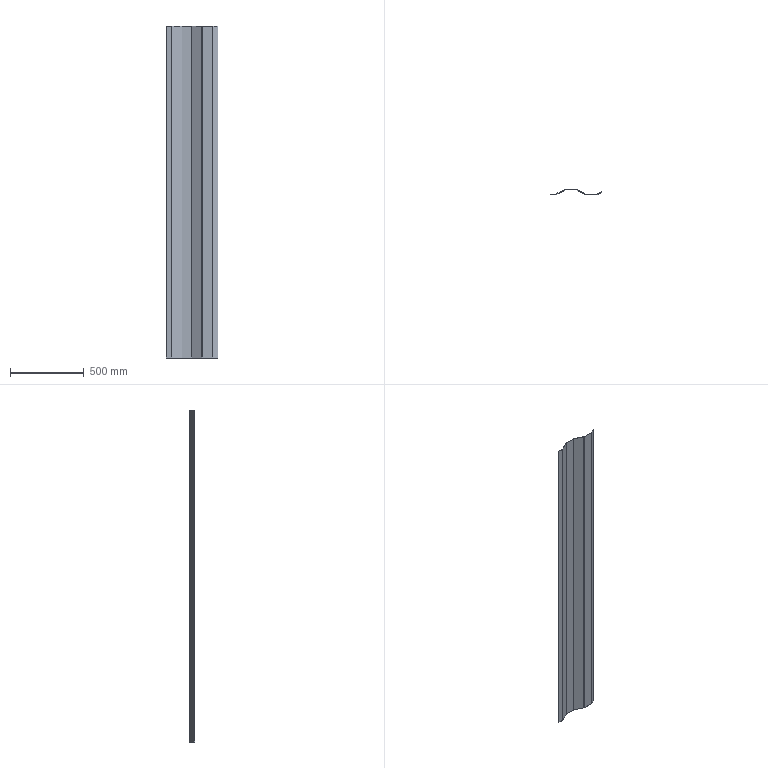Part | STEP file | 750078174 | 1 solid | 26 faces | box 347 x 36 x 2253 mm | volume 1650208 mm3 | plane 16 | cylinder 10 | commonest cylinder face diameters 6 x5 10 x5
STEP:
#1=CARTESIAN_POINT('',(102.472,35.472,0.));
#2=VERTEX_POINT('',#1);
#3=CARTESIAN_POINT('',(36.161,2.317,0.));
#4=VERTEX_POINT('',#3);
#5=CARTESIAN_POINT('',(103.106,35.789,0.));
#6=DIRECTION('',(-0.8944,-0.4472,0.));
#7=VECTOR('',#6,1000.);
#8=LINE('',#5,#7);
#9=EDGE_CURVE('',#2,#4,#8,.T.);
#10=ORIENTED_EDGE('',*,*,#9,.T.);
#11=CARTESIAN_POINT('',(36.161,2.317,2252.5));
#12=VERTEX_POINT('',#11);
#13=CARTESIAN_POINT('',(36.161,2.317,0.));
#14=DIRECTION('',(0.,0.,1.));
#15=VECTOR('',#14,1000.);
#16=LINE('',#13,#15);
#17=EDGE_CURVE('',#4,#12,#16,.T.);
#18=ORIENTED_EDGE('',*,*,#17,.T.);
#19=CARTESIAN_POINT('',(102.472,35.472,2252.5));
#20=VERTEX_POINT('',#19);
#21=CARTESIAN_POINT('',(103.106,35.789,2252.5));
#22=DIRECTION('',(0.8944,0.4472,0.));
#23=VECTOR('',#22,1000.);
#24=LINE('',#21,#23);
#25=EDGE_CURVE('',#12,#20,#24,.T.);
#26=ORIENTED_EDGE('',*,*,#25,.T.);
#27=CARTESIAN_POINT('',(102.472,35.472,0.));
#28=DIRECTION('',(0.,0.,-1.));
#29=VECTOR('',#28,1000.);
#30=LINE('',#27,#29);
#31=EDGE_CURVE('',#20,#2,#30,.T.);
#32=ORIENTED_EDGE('',*,*,#31,.T.);
#33=EDGE_LOOP('',(#10,#18,#26,#32));
#34=FACE_OUTER_BOUND('',#33,.T.);
#35=CARTESIAN_POINT('',(103.106,35.789,0.));
#36=DIRECTION('',(-0.4472,0.8944,0.));
#37=DIRECTION('',(-0.8944,-0.4472,0.));
#38=AXIS2_PLACEMENT_3D('',#35,#36,#37);
#39=PLANE('',#38);
#40=ADVANCED_FACE('',(#34),#39,.T.);
#41=ORIENTED_EDGE('',*,*,#17,.F.);
#42=CARTESIAN_POINT('',(34.82,2.,0.));
#43=VERTEX_POINT('',#42);
#44=CARTESIAN_POINT('',(34.82,5.,0.));
#45=DIRECTION('',(0.,0.,1.));
#46=DIRECTION('',(1.,0.,0.));
#47=AXIS2_PLACEMENT_3D('',#44,#45,#46);
#48=CIRCLE('',#47,3.);
#49=EDGE_CURVE('',#43,#4,#48,.T.);
#50=ORIENTED_EDGE('',*,*,#49,.F.);
#51=CARTESIAN_POINT('',(34.82,2.,2252.5));
#52=VERTEX_POINT('',#51);
#53=CARTESIAN_POINT('',(34.82,2.,0.));
#54=DIRECTION('',(0.,0.,-1.));
#55=VECTOR('',#54,1000.);
#56=LINE('',#53,#55);
#57=EDGE_CURVE('',#52,#43,#56,.T.);
#58=ORIENTED_EDGE('',*,*,#57,.F.);
#59=CARTESIAN_POINT('',(34.82,5.,2252.5));
#60=DIRECTION('',(0.,0.,-1.));
#61=DIRECTION('',(1.,0.,0.));
#62=AXIS2_PLACEMENT_3D('',#59,#60,#61);
#63=CIRCLE('',#62,3.);
#64=EDGE_CURVE('',#12,#52,#63,.T.);
#65=ORIENTED_EDGE('',*,*,#64,.F.);
#66=EDGE_LOOP('',(#41,#50,#58,#65));
#67=FACE_OUTER_BOUND('',#66,.T.);
#68=CARTESIAN_POINT('',(34.82,5.,0.));
#69=DIRECTION('',(0.,0.,1.));
#70=DIRECTION('',(1.,0.,0.));
#71=AXIS2_PLACEMENT_3D('',#68,#69,#70);
#72=CYLINDRICAL_SURFACE('',#71,3.);
#73=ADVANCED_FACE('',(#67),#72,.F.);
#74=CARTESIAN_POINT('',(314.161,2.317,0.));
#75=VERTEX_POINT('',#74);
#76=CARTESIAN_POINT('',(346.106,18.289,0.));
#77=VERTEX_POINT('',#76);
#78=CARTESIAN_POINT('',(314.161,2.317,0.));
#79=DIRECTION('',(0.8944,0.4472,0.));
#80=VECTOR('',#79,1000.);
#81=LINE('',#78,#80);
#82=EDGE_CURVE('',#75,#77,#81,.T.);
#83=ORIENTED_EDGE('',*,*,#82,.T.);
#84=CARTESIAN_POINT('',(347.,16.5,0.));
#85=VERTEX_POINT('',#84);
#86=CARTESIAN_POINT('',(346.106,18.289,0.));
#87=DIRECTION('',(0.4472,-0.8944,0.));
#88=VECTOR('',#87,1000.);
#89=LINE('',#86,#88);
#90=EDGE_CURVE('',#77,#85,#89,.T.);
#91=ORIENTED_EDGE('',*,*,#90,.T.);
#92=CARTESIAN_POINT('',(315.056,0.5279,0.));
#93=VERTEX_POINT('',#92);
#94=CARTESIAN_POINT('',(347.,16.5,0.));
#95=DIRECTION('',(-0.8944,-0.4472,0.));
#96=VECTOR('',#95,1000.);
#97=LINE('',#94,#96);
#98=EDGE_CURVE('',#85,#93,#97,.T.);
#99=ORIENTED_EDGE('',*,*,#98,.T.);
#100=CARTESIAN_POINT('',(312.82,0.,0.));
#101=VERTEX_POINT('',#100);
#102=CARTESIAN_POINT('',(312.82,5.,0.));
#103=DIRECTION('',(0.,0.,-1.));
#104=DIRECTION('',(1.,0.,0.));
#105=AXIS2_PLACEMENT_3D('',#102,#103,#104);
#106=CIRCLE('',#105,5.);
#107=EDGE_CURVE('',#93,#101,#106,.T.);
#108=ORIENTED_EDGE('',*,*,#107,.T.);
#109=CARTESIAN_POINT('',(243.18,0.,0.));
#110=VERTEX_POINT('',#109);
#111=CARTESIAN_POINT('',(347.,0.,0.));
#112=DIRECTION('',(-1.,0.,0.));
#113=VECTOR('',#112,1000.);
#114=LINE('',#111,#113);
#115=EDGE_CURVE('',#101,#110,#114,.T.);
#116=ORIENTED_EDGE('',*,*,#115,.T.);
#117=CARTESIAN_POINT('',(240.944,0.5279,0.));
#118=VERTEX_POINT('',#117);
#119=CARTESIAN_POINT('',(243.18,5.,0.));
#120=DIRECTION('',(0.,0.,-1.));
#121=DIRECTION('',(1.,0.,0.));
#122=AXIS2_PLACEMENT_3D('',#119,#120,#121);
#123=CIRCLE('',#122,5.);
#124=EDGE_CURVE('',#110,#118,#123,.T.);
#125=ORIENTED_EDGE('',*,*,#124,.T.);
#126=CARTESIAN_POINT('',(174.633,33.683,0.));
#127=VERTEX_POINT('',#126);
#128=CARTESIAN_POINT('',(240.944,0.5279,0.));
#129=DIRECTION('',(-0.8944,0.4472,0.));
#130=VECTOR('',#129,1000.);
#131=LINE('',#128,#130);
#132=EDGE_CURVE('',#118,#127,#131,.T.);
#133=ORIENTED_EDGE('',*,*,#132,.T.);
#134=CARTESIAN_POINT('',(173.292,34.,0.));
#135=VERTEX_POINT('',#134);
#136=CARTESIAN_POINT('',(173.292,31.,0.));
#137=DIRECTION('',(0.,0.,1.));
#138=DIRECTION('',(1.,0.,0.));
#139=AXIS2_PLACEMENT_3D('',#136,#137,#138);
#140=CIRCLE('',#139,3.);
#141=EDGE_CURVE('',#127,#135,#140,.T.);
#142=ORIENTED_EDGE('',*,*,#141,.T.);
#143=CARTESIAN_POINT('',(104.708,34.,0.));
#144=VERTEX_POINT('',#143);
#145=CARTESIAN_POINT('',(347.,34.,0.));
#146=DIRECTION('',(-1.,0.,0.));
#147=VECTOR('',#146,1000.);
#148=LINE('',#145,#147);
#149=EDGE_CURVE('',#135,#144,#148,.T.);
#150=ORIENTED_EDGE('',*,*,#149,.T.);
#151=CARTESIAN_POINT('',(103.367,33.683,0.));
#152=VERTEX_POINT('',#151);
#153=CARTESIAN_POINT('',(104.708,31.,0.));
#154=DIRECTION('',(0.,0.,1.));
#155=DIRECTION('',(1.,0.,0.));
#156=AXIS2_PLACEMENT_3D('',#153,#154,#155);
#157=CIRCLE('',#156,3.);
#158=EDGE_CURVE('',#144,#152,#157,.T.);
#159=ORIENTED_EDGE('',*,*,#158,.T.);
#160=CARTESIAN_POINT('',(37.056,0.5279,0.));
#161=VERTEX_POINT('',#160);
#162=CARTESIAN_POINT('',(103.367,33.683,0.));
#163=DIRECTION('',(-0.8944,-0.4472,0.));
#164=VECTOR('',#163,1000.);
#165=LINE('',#162,#164);
#166=EDGE_CURVE('',#152,#161,#165,.T.);
#167=ORIENTED_EDGE('',*,*,#166,.T.);
#168=CARTESIAN_POINT('',(34.82,0.,0.));
#169=VERTEX_POINT('',#168);
#170=CARTESIAN_POINT('',(34.82,5.,0.));
#171=DIRECTION('',(0.,0.,-1.));
#172=DIRECTION('',(1.,0.,0.));
#173=AXIS2_PLACEMENT_3D('',#170,#171,#172);
#174=CIRCLE('',#173,5.);
#175=EDGE_CURVE('',#161,#169,#174,.T.);
#176=ORIENTED_EDGE('',*,*,#175,.T.);
#177=CARTESIAN_POINT('',(0.,0.,0.));
#178=VERTEX_POINT('',#177);
#179=CARTESIAN_POINT('',(347.,0.,0.));
#180=DIRECTION('',(-1.,0.,0.));
#181=VECTOR('',#180,1000.);
#182=LINE('',#179,#181);
#183=EDGE_CURVE('',#169,#178,#182,.T.);
#184=ORIENTED_EDGE('',*,*,#183,.T.);
#185=CARTESIAN_POINT('',(0.,2.,0.));
#186=VERTEX_POINT('',#185);
#187=CARTESIAN_POINT('',(0.,16.5,0.));
#188=DIRECTION('',(0.,1.,0.));
#189=VECTOR('',#188,1000.);
#190=LINE('',#187,#189);
#191=EDGE_CURVE('',#178,#186,#190,.T.);
#192=ORIENTED_EDGE('',*,*,#191,.T.);
#193=CARTESIAN_POINT('',(347.,2.,0.));
#194=DIRECTION('',(1.,0.,0.));
#195=VECTOR('',#194,1000.);
#196=LINE('',#193,#195);
#197=EDGE_CURVE('',#186,#43,#196,.T.);
#198=ORIENTED_EDGE('',*,*,#197,.T.);
#199=ORIENTED_EDGE('',*,*,#49,.T.);
#200=ORIENTED_EDGE('',*,*,#9,.F.);
#201=CARTESIAN_POINT('',(104.708,36.,0.));
#202=VERTEX_POINT('',#201);
#203=CARTESIAN_POINT('',(104.708,31.,0.));
#204=DIRECTION('',(0.,0.,-1.));
#205=DIRECTION('',(1.,0.,0.));
#206=AXIS2_PLACEMENT_3D('',#203,#204,#205);
#207=CIRCLE('',#206,5.);
#208=EDGE_CURVE('',#2,#202,#207,.T.);
#209=ORIENTED_EDGE('',*,*,#208,.T.);
#210=CARTESIAN_POINT('',(173.292,36.,0.));
#211=VERTEX_POINT('',#210);
#212=CARTESIAN_POINT('',(347.,36.,0.));
#213=DIRECTION('',(1.,0.,0.));
#214=VECTOR('',#213,1000.);
#215=LINE('',#212,#214);
#216=EDGE_CURVE('',#202,#211,#215,.T.);
#217=ORIENTED_EDGE('',*,*,#216,.T.);
#218=CARTESIAN_POINT('',(175.528,35.472,0.));
#219=VERTEX_POINT('',#218);
#220=CARTESIAN_POINT('',(173.292,31.,0.));
#221=DIRECTION('',(0.,0.,-1.));
#222=DIRECTION('',(1.,0.,0.));
#223=AXIS2_PLACEMENT_3D('',#220,#221,#222);
#224=CIRCLE('',#223,5.);
#225=EDGE_CURVE('',#211,#219,#224,.T.);
#226=ORIENTED_EDGE('',*,*,#225,.T.);
#227=CARTESIAN_POINT('',(241.839,2.317,0.));
#228=VERTEX_POINT('',#227);
#229=CARTESIAN_POINT('',(175.528,35.472,0.));
#230=DIRECTION('',(0.8944,-0.4472,0.));
#231=VECTOR('',#230,1000.);
#232=LINE('',#229,#231);
#233=EDGE_CURVE('',#219,#228,#232,.T.);
#234=ORIENTED_EDGE('',*,*,#233,.T.);
#235=CARTESIAN_POINT('',(243.18,2.,0.));
#236=VERTEX_POINT('',#235);
#237=CARTESIAN_POINT('',(243.18,5.,0.));
#238=DIRECTION('',(0.,0.,1.));
#239=DIRECTION('',(1.,0.,0.));
#240=AXIS2_PLACEMENT_3D('',#237,#238,#239);
#241=CIRCLE('',#240,3.);
#242=EDGE_CURVE('',#228,#236,#241,.T.);
#243=ORIENTED_EDGE('',*,*,#242,.T.);
#244=CARTESIAN_POINT('',(312.82,2.,0.));
#245=VERTEX_POINT('',#244);
#246=CARTESIAN_POINT('',(347.,2.,0.));
#247=DIRECTION('',(1.,0.,0.));
#248=VECTOR('',#247,1000.);
#249=LINE('',#246,#248);
#250=EDGE_CURVE('',#236,#245,#249,.T.);
#251=ORIENTED_EDGE('',*,*,#250,.T.);
#252=CARTESIAN_POINT('',(312.82,5.,0.));
#253=DIRECTION('',(0.,0.,1.));
#254=DIRECTION('',(1.,0.,0.));
#255=AXIS2_PLACEMENT_3D('',#252,#253,#254);
#256=CIRCLE('',#255,3.);
#257=EDGE_CURVE('',#245,#75,#256,.T.);
#258=ORIENTED_EDGE('',*,*,#257,.T.);
#259=EDGE_LOOP('',(#83,#91,#99,#108,#116,#125,#133,#142,#150,#159,#167,#176,#184,#192,#198,#199,#200,#209,#217,#226,#234,#243,#251,#258));
#260=FACE_OUTER_BOUND('',#259,.T.);
#261=CARTESIAN_POINT('',(347.,16.5,0.));
#262=DIRECTION('',(0.,0.,-1.));
#263=DIRECTION('',(-1.,0.,0.));
#264=AXIS2_PLACEMENT_3D('',#261,#262,#263);
#265=PLANE('',#264);
#266=ADVANCED_FACE('',(#260),#265,.T.);
#267=ORIENTED_EDGE('',*,*,#208,.F.);
#268=ORIENTED_EDGE('',*,*,#31,.F.);
#269=CARTESIAN_POINT('',(104.708,36.,2252.5));
#270=VERTEX_POINT('',#269);
#271=CARTESIAN_POINT('',(104.708,31.,2252.5));
#272=DIRECTION('',(0.,0.,-1.));
#273=DIRECTION('',(1.,0.,0.));
#274=AXIS2_PLACEMENT_3D('',#271,#272,#273);
#275=CIRCLE('',#274,5.);
#276=EDGE_CURVE('',#20,#270,#275,.T.);
#277=ORIENTED_EDGE('',*,*,#276,.T.);
#278=CARTESIAN_POINT('',(104.708,36.,0.));
#279=DIRECTION('',(0.,0.,-1.));
#280=VECTOR('',#279,1000.);
#281=LINE('',#278,#280);
#282=EDGE_CURVE('',#270,#202,#281,.T.);
#283=ORIENTED_EDGE('',*,*,#282,.T.);
#284=EDGE_LOOP('',(#267,#268,#277,#283));
#285=FACE_OUTER_BOUND('',#284,.T.);
#286=CARTESIAN_POINT('',(104.708,31.,0.));
#287=DIRECTION('',(0.,0.,1.));
#288=DIRECTION('',(1.,0.,0.));
#289=AXIS2_PLACEMENT_3D('',#286,#287,#288);
#290=CYLINDRICAL_SURFACE('',#289,5.);
#291=ADVANCED_FACE('',(#285),#290,.T.);
#292=CARTESIAN_POINT('',(243.18,2.,2252.5));
#293=VERTEX_POINT('',#292);
#294=CARTESIAN_POINT('',(312.82,2.,2252.5));
#295=VERTEX_POINT('',#294);
#296=CARTESIAN_POINT('',(312.82,2.,2252.5));
#297=DIRECTION('',(1.,0.,0.));
#298=VECTOR('',#297,1000.);
#299=LINE('',#296,#298);
#300=EDGE_CURVE('',#293,#295,#299,.T.);
#301=ORIENTED_EDGE('',*,*,#300,.F.);
#302=CARTESIAN_POINT('',(241.839,2.317,2252.5));
#303=VERTEX_POINT('',#302);
#304=CARTESIAN_POINT('',(243.18,5.,2252.5));
#305=DIRECTION('',(0.,0.,-1.));
#306=DIRECTION('',(1.,0.,0.));
#307=AXIS2_PLACEMENT_3D('',#304,#305,#306);
#308=CIRCLE('',#307,3.);
#309=EDGE_CURVE('',#293,#303,#308,.T.);
#310=ORIENTED_EDGE('',*,*,#309,.T.);
#311=CARTESIAN_POINT('',(175.528,35.472,2252.5));
#312=VERTEX_POINT('',#311);
#313=CARTESIAN_POINT('',(175.528,35.472,2252.5));
#314=DIRECTION('',(0.8944,-0.4472,0.));
#315=VECTOR('',#314,1000.);
#316=LINE('',#313,#315);
#317=EDGE_CURVE('',#312,#303,#316,.T.);
#318=ORIENTED_EDGE('',*,*,#317,.F.);
#319=CARTESIAN_POINT('',(173.292,36.,2252.5));
#320=VERTEX_POINT('',#319);
#321=CARTESIAN_POINT('',(173.292,31.,2252.5));
#322=DIRECTION('',(0.,0.,-1.));
#323=DIRECTION('',(1.,0.,0.));
#324=AXIS2_PLACEMENT_3D('',#321,#322,#323);
#325=CIRCLE('',#324,5.);
#326=EDGE_CURVE('',#320,#312,#325,.T.);
#327=ORIENTED_EDGE('',*,*,#326,.F.);
#328=CARTESIAN_POINT('',(312.82,36.,2252.5));
#329=DIRECTION('',(1.,0.,0.));
#330=VECTOR('',#329,1000.);
#331=LINE('',#328,#330);
#332=EDGE_CURVE('',#270,#320,#331,.T.);
#333=ORIENTED_EDGE('',*,*,#332,.F.);
#334=ORIENTED_EDGE('',*,*,#276,.F.);
#335=ORIENTED_EDGE('',*,*,#25,.F.);
#336=ORIENTED_EDGE('',*,*,#64,.T.);
#337=CARTESIAN_POINT('',(0.,2.,2252.5));
#338=VERTEX_POINT('',#337);
#339=CARTESIAN_POINT('',(312.82,2.,2252.5));
#340=DIRECTION('',(1.,0.,0.));
#341=VECTOR('',#340,1000.);
#342=LINE('',#339,#341);
#343=EDGE_CURVE('',#338,#52,#342,.T.);
#344=ORIENTED_EDGE('',*,*,#343,.F.);
#345=CARTESIAN_POINT('',(0.,0.,2252.5));
#346=VERTEX_POINT('',#345);
#347=CARTESIAN_POINT('',(0.,5.,2252.5));
#348=DIRECTION('',(0.,1.,0.));
#349=VECTOR('',#348,1000.);
#350=LINE('',#347,#349);
#351=EDGE_CURVE('',#346,#338,#350,.T.);
#352=ORIENTED_EDGE('',*,*,#351,.F.);
#353=CARTESIAN_POINT('',(34.82,0.,2252.5));
#354=VERTEX_POINT('',#353);
#355=CARTESIAN_POINT('',(312.82,0.,2252.5));
#356=DIRECTION('',(-1.,0.,0.));
#357=VECTOR('',#356,1000.);
#358=LINE('',#355,#357);
#359=EDGE_CURVE('',#354,#346,#358,.T.);
#360=ORIENTED_EDGE('',*,*,#359,.F.);
#361=CARTESIAN_POINT('',(37.056,0.5279,2252.5));
#362=VERTEX_POINT('',#361);
#363=CARTESIAN_POINT('',(34.82,5.,2252.5));
#364=DIRECTION('',(0.,0.,-1.));
#365=DIRECTION('',(1.,0.,0.));
#366=AXIS2_PLACEMENT_3D('',#363,#364,#365);
#367=CIRCLE('',#366,5.);
#368=EDGE_CURVE('',#362,#354,#367,.T.);
#369=ORIENTED_EDGE('',*,*,#368,.F.);
#370=CARTESIAN_POINT('',(103.367,33.683,2252.5));
#371=VERTEX_POINT('',#370);
#372=CARTESIAN_POINT('',(103.367,33.683,2252.5));
#373=DIRECTION('',(-0.8944,-0.4472,0.));
#374=VECTOR('',#373,1000.);
#375=LINE('',#372,#374);
#376=EDGE_CURVE('',#371,#362,#375,.T.);
#377=ORIENTED_EDGE('',*,*,#376,.F.);
#378=CARTESIAN_POINT('',(104.708,34.,2252.5));
#379=VERTEX_POINT('',#378);
#380=CARTESIAN_POINT('',(104.708,31.,2252.5));
#381=DIRECTION('',(0.,0.,-1.));
#382=DIRECTION('',(1.,0.,0.));
#383=AXIS2_PLACEMENT_3D('',#380,#381,#382);
#384=CIRCLE('',#383,3.);
#385=EDGE_CURVE('',#371,#379,#384,.T.);
#386=ORIENTED_EDGE('',*,*,#385,.T.);
#387=CARTESIAN_POINT('',(173.292,34.,2252.5));
#388=VERTEX_POINT('',#387);
#389=CARTESIAN_POINT('',(312.82,34.,2252.5));
#390=DIRECTION('',(-1.,0.,0.));
#391=VECTOR('',#390,1000.);
#392=LINE('',#389,#391);
#393=EDGE_CURVE('',#388,#379,#392,.T.);
#394=ORIENTED_EDGE('',*,*,#393,.F.);
#395=CARTESIAN_POINT('',(174.633,33.683,2252.5));
#396=VERTEX_POINT('',#395);
#397=CARTESIAN_POINT('',(173.292,31.,2252.5));
#398=DIRECTION('',(0.,0.,-1.));
#399=DIRECTION('',(1.,0.,0.));
#400=AXIS2_PLACEMENT_3D('',#397,#398,#399);
#401=CIRCLE('',#400,3.);
#402=EDGE_CURVE('',#388,#396,#401,.T.);
#403=ORIENTED_EDGE('',*,*,#402,.T.);
#404=CARTESIAN_POINT('',(240.944,0.5279,2252.5));
#405=VERTEX_POINT('',#404);
#406=CARTESIAN_POINT('',(240.944,0.5279,2252.5));
#407=DIRECTION('',(-0.8944,0.4472,0.));
#408=VECTOR('',#407,1000.);
#409=LINE('',#406,#408);
#410=EDGE_CURVE('',#405,#396,#409,.T.);
#411=ORIENTED_EDGE('',*,*,#410,.F.);
#412=CARTESIAN_POINT('',(243.18,0.,2252.5));
#413=VERTEX_POINT('',#412);
#414=CARTESIAN_POINT('',(243.18,5.,2252.5));
#415=DIRECTION('',(0.,0.,-1.));
#416=DIRECTION('',(1.,0.,0.));
#417=AXIS2_PLACEMENT_3D('',#414,#415,#416);
#418=CIRCLE('',#417,5.);
#419=EDGE_CURVE('',#413,#405,#418,.T.);
#420=ORIENTED_EDGE('',*,*,#419,.F.);
#421=CARTESIAN_POINT('',(312.82,0.,2252.5));
#422=VERTEX_POINT('',#421);
#423=CARTESIAN_POINT('',(312.82,0.,2252.5));
#424=DIRECTION('',(-1.,0.,0.));
#425=VECTOR('',#424,1000.);
#426=LINE('',#423,#425);
#427=EDGE_CURVE('',#422,#413,#426,.T.);
#428=ORIENTED_EDGE('',*,*,#427,.F.);
#429=CARTESIAN_POINT('',(315.056,0.5279,2252.5));
#430=VERTEX_POINT('',#429);
#431=CARTESIAN_POINT('',(312.82,5.,2252.5));
#432=DIRECTION('',(0.,0.,-1.));
#433=DIRECTION('',(1.,0.,0.));
#434=AXIS2_PLACEMENT_3D('',#431,#432,#433);
#435=CIRCLE('',#434,5.);
#436=EDGE_CURVE('',#430,#422,#435,.T.);
#437=ORIENTED_EDGE('',*,*,#436,.F.);
#438=CARTESIAN_POINT('',(347.,16.5,2252.5));
#439=VERTEX_POINT('',#438);
#440=CARTESIAN_POINT('',(347.,16.5,2252.5));
#441=DIRECTION('',(-0.8944,-0.4472,0.));
#442=VECTOR('',#441,1000.);
#443=LINE('',#440,#442);
#444=EDGE_CURVE('',#439,#430,#443,.T.);
#445=ORIENTED_EDGE('',*,*,#444,.F.);
#446=CARTESIAN_POINT('',(346.106,18.289,2252.5));
#447=VERTEX_POINT('',#446);
#448=CARTESIAN_POINT('',(346.106,18.289,2252.5));
#449=DIRECTION('',(0.4472,-0.8944,0.));
#450=VECTOR('',#449,1000.);
#451=LINE('',#448,#450);
#452=EDGE_CURVE('',#447,#439,#451,.T.);
#453=ORIENTED_EDGE('',*,*,#452,.F.);
#454=CARTESIAN_POINT('',(314.161,2.317,2252.5));
#455=VERTEX_POINT('',#454);
#456=CARTESIAN_POINT('',(314.161,2.317,2252.5));
#457=DIRECTION('',(0.8944,0.4472,0.));
#458=VECTOR('',#457,1000.);
#459=LINE('',#456,#458);
#460=EDGE_CURVE('',#455,#447,#459,.T.);
#461=ORIENTED_EDGE('',*,*,#460,.F.);
#462=CARTESIAN_POINT('',(312.82,5.,2252.5));
#463=DIRECTION('',(0.,0.,-1.));
#464=DIRECTION('',(1.,0.,0.));
#465=AXIS2_PLACEMENT_3D('',#462,#463,#464);
#466=CIRCLE('',#465,3.);
#467=EDGE_CURVE('',#455,#295,#466,.T.);
#468=ORIENTED_EDGE('',*,*,#467,.T.);
#469=EDGE_LOOP('',(#301,#310,#318,#327,#333,#334,#335,#336,#344,#352,#360,#369,#377,#386,#394,#403,#411,#420,#428,#437,#445,#453,#461,#468));
#470=FACE_OUTER_BOUND('',#469,.T.);
#471=CARTESIAN_POINT('',(312.82,5.,2252.5));
#472=DIRECTION('',(0.,0.,-1.));
#473=DIRECTION('',(-1.,0.,0.));
#474=AXIS2_PLACEMENT_3D('',#471,#472,#473);
#475=PLANE('',#474);
#476=ADVANCED_FACE('',(#470),#475,.F.);
#477=ORIENTED_EDGE('',*,*,#197,.F.);
#478=CARTESIAN_POINT('',(0.,2.,0.));
#479=DIRECTION('',(0.,0.,1.));
#480=VECTOR('',#479,1000.);
#481=LINE('',#478,#480);
#482=EDGE_CURVE('',#186,#338,#481,.T.);
#483=ORIENTED_EDGE('',*,*,#482,.T.);
#484=ORIENTED_EDGE('',*,*,#343,.T.);
#485=ORIENTED_EDGE('',*,*,#57,.T.);
#486=EDGE_LOOP('',(#477,#483,#484,#485));
#487=FACE_OUTER_BOUND('',#486,.T.);
#488=CARTESIAN_POINT('',(36.,2.,0.));
#489=DIRECTION('',(0.,1.,0.));
#490=DIRECTION('',(-1.,0.,0.));
#491=AXIS2_PLACEMENT_3D('',#488,#489,#490);
#492=PLANE('',#491);
#493=ADVANCED_FACE('',(#487),#492,.T.);
#494=CARTESIAN_POINT('',(346.106,18.289,0.));
#495=DIRECTION('',(0.,0.,-1.));
#496=VECTOR('',#495,1000.);
#497=LINE('',#494,#496);
#498=EDGE_CURVE('',#447,#77,#497,.T.);
#499=ORIENTED_EDGE('',*,*,#498,.F.);
#500=ORIENTED_EDGE('',*,*,#452,.T.);
#501=CARTESIAN_POINT('',(347.,16.5,0.));
#502=DIRECTION('',(0.,0.,1.));
#503=VECTOR('',#502,1000.);
#504=LINE('',#501,#503);
#505=EDGE_CURVE('',#85,#439,#504,.T.);
#506=ORIENTED_EDGE('',*,*,#505,.F.);
#507=ORIENTED_EDGE('',*,*,#90,.F.);
#508=EDGE_LOOP('',(#499,#500,#506,#507));
#509=FACE_OUTER_BOUND('',#508,.T.);
#510=CARTESIAN_POINT('',(347.,16.5,0.));
#511=DIRECTION('',(-0.8944,-0.4472,0.));
#512=DIRECTION('',(0.4472,-0.8944,0.));
#513=AXIS2_PLACEMENT_3D('',#510,#511,#512);
#514=PLANE('',#513);
#515=ADVANCED_FACE('',(#509),#514,.F.);
#516=ORIENTED_EDGE('',*,*,#82,.F.);
#517=CARTESIAN_POINT('',(314.161,2.317,0.));
#518=DIRECTION('',(0.,0.,1.));
#519=VECTOR('',#518,1000.);
#520=LINE('',#517,#519);
#521=EDGE_CURVE('',#75,#455,#520,.T.);
#522=ORIENTED_EDGE('',*,*,#521,.T.);
#523=ORIENTED_EDGE('',*,*,#460,.T.);
#524=ORIENTED_EDGE('',*,*,#498,.T.);
#525=EDGE_LOOP('',(#516,#522,#523,#524));
#526=FACE_OUTER_BOUND('',#525,.T.);
#527=CARTESIAN_POINT('',(346.106,18.289,0.));
#528=DIRECTION('',(-0.4472,0.8944,0.));
#529=DIRECTION('',(-0.8944,-0.4472,0.));
#530=AXIS2_PLACEMENT_3D('',#527,#528,#529);
#531=PLANE('',#530);
#532=ADVANCED_FACE('',(#526),#531,.T.);
#533=ORIENTED_EDGE('',*,*,#250,.F.);
#534=CARTESIAN_POINT('',(243.18,2.,0.));
#535=DIRECTION('',(0.,0.,1.));
#536=VECTOR('',#535,1000.);
#537=LINE('',#534,#536);
#538=EDGE_CURVE('',#236,#293,#537,.T.);
#539=ORIENTED_EDGE('',*,*,#538,.T.);
#540=ORIENTED_EDGE('',*,*,#300,.T.);
#541=CARTESIAN_POINT('',(312.82,2.,0.));
#542=DIRECTION('',(0.,0.,-1.));
#543=VECTOR('',#542,1000.);
#544=LINE('',#541,#543);
#545=EDGE_CURVE('',#295,#245,#544,.T.);
#546=ORIENTED_EDGE('',*,*,#545,.T.);
#547=EDGE_LOOP('',(#533,#539,#540,#546));
#548=FACE_OUTER_BOUND('',#547,.T.);
#549=CARTESIAN_POINT('',(314.,2.,0.));
#550=DIRECTION('',(0.,1.,0.));
#551=DIRECTION('',(0.,0.,1.));
#552=AXIS2_PLACEMENT_3D('',#549,#550,#551);
#553=PLANE('',#552);
#554=ADVANCED_FACE('',(#548),#553,.T.);
#555=ORIENTED_EDGE('',*,*,#233,.F.);
#556=CARTESIAN_POINT('',(175.528,35.472,0.));
#557=DIRECTION('',(0.,0.,1.));
#558=VECTOR('',#557,1000.);
#559=LINE('',#556,#558);
#560=EDGE_CURVE('',#219,#312,#559,.T.);
#561=ORIENTED_EDGE('',*,*,#560,.T.);
#562=ORIENTED_EDGE('',*,*,#317,.T.);
#563=CARTESIAN_POINT('',(241.839,2.317,0.));
#564=DIRECTION('',(0.,0.,-1.));
#565=VECTOR('',#564,1000.);
#566=LINE('',#563,#565);
#567=EDGE_CURVE('',#303,#228,#566,.T.);
#568=ORIENTED_EDGE('',*,*,#567,.T.);
#569=EDGE_LOOP('',(#555,#561,#562,#568));
#570=FACE_OUTER_BOUND('',#569,.T.);
#571=CARTESIAN_POINT('',(242.894,1.789,0.));
#572=DIRECTION('',(0.4472,0.8944,0.));
#573=DIRECTION('',(-0.8944,0.4472,0.));
#574=AXIS2_PLACEMENT_3D('',#571,#572,#573);
#575=PLANE('',#574);
#576=ADVANCED_FACE('',(#570),#575,.T.);
#577=ORIENTED_EDGE('',*,*,#225,.F.);
#578=CARTESIAN_POINT('',(173.292,36.,0.));
#579=DIRECTION('',(0.,0.,1.));
#580=VECTOR('',#579,1000.);
#581=LINE('',#578,#580);
#582=EDGE_CURVE('',#211,#320,#581,.T.);
#583=ORIENTED_EDGE('',*,*,#582,.T.);
#584=ORIENTED_EDGE('',*,*,#326,.T.);
#585=ORIENTED_EDGE('',*,*,#560,.F.);
#586=EDGE_LOOP('',(#577,#583,#584,#585));
#587=FACE_OUTER_BOUND('',#586,.T.);
#588=CARTESIAN_POINT('',(173.292,31.,0.));
#589=DIRECTION('',(0.,0.,1.));
#590=DIRECTION('',(1.,0.,0.));
#591=AXIS2_PLACEMENT_3D('',#588,#589,#590);
#592=CYLINDRICAL_SURFACE('',#591,5.);
#593=ADVANCED_FACE('',(#587),#592,.T.);
#594=ORIENTED_EDGE('',*,*,#216,.F.);
#595=ORIENTED_EDGE('',*,*,#282,.F.);
#596=ORIENTED_EDGE('',*,*,#332,.T.);
#597=ORIENTED_EDGE('',*,*,#582,.F.);
#598=EDGE_LOOP('',(#594,#595,#596,#597));
#599=FACE_OUTER_BOUND('',#598,.T.);
#600=CARTESIAN_POINT('',(174.,36.,0.));
#601=DIRECTION('',(0.,1.,0.));
#602=DIRECTION('',(0.,0.,1.));
#603=AXIS2_PLACEMENT_3D('',#600,#601,#602);
#604=PLANE('',#603);
#605=ADVANCED_FACE('',(#599),#604,.T.);
#606=ORIENTED_EDGE('',*,*,#191,.F.);
#607=CARTESIAN_POINT('',(0.,0.,0.));
#608=DIRECTION('',(0.,0.,1.));
#609=VECTOR('',#608,1000.);
#610=LINE('',#607,#609);
#611=EDGE_CURVE('',#178,#346,#610,.T.);
#612=ORIENTED_EDGE('',*,*,#611,.T.);
#613=ORIENTED_EDGE('',*,*,#351,.T.);
#614=ORIENTED_EDGE('',*,*,#482,.F.);
#615=EDGE_LOOP('',(#606,#612,#613,#614));
#616=FACE_OUTER_BOUND('',#615,.T.);
#617=CARTESIAN_POINT('',(0.,0.,0.));
#618=DIRECTION('',(-1.,0.,0.));
#619=DIRECTION('',(0.,-1.,0.));
#620=AXIS2_PLACEMENT_3D('',#617,#618,#619);
#621=PLANE('',#620);
#622=ADVANCED_FACE('',(#616),#621,.T.);
#623=ORIENTED_EDGE('',*,*,#611,.F.);
#624=ORIENTED_EDGE('',*,*,#183,.F.);
#625=CARTESIAN_POINT('',(34.82,0.,0.));
#626=DIRECTION('',(0.,0.,-1.));
#627=VECTOR('',#626,1000.);
#628=LINE('',#625,#627);
#629=EDGE_CURVE('',#354,#169,#628,.T.);
#630=ORIENTED_EDGE('',*,*,#629,.F.);
#631=ORIENTED_EDGE('',*,*,#359,.T.);
#632=EDGE_LOOP('',(#623,#624,#630,#631));
#633=FACE_OUTER_BOUND('',#632,.T.);
#634=CARTESIAN_POINT('',(36.,0.,0.));
#635=DIRECTION('',(0.,1.,0.));
#636=DIRECTION('',(-1.,0.,0.));
#637=AXIS2_PLACEMENT_3D('',#634,#635,#636);
#638=PLANE('',#637);
#639=ADVANCED_FACE('',(#633),#638,.F.);
#640=ORIENTED_EDGE('',*,*,#175,.F.);
#641=CARTESIAN_POINT('',(37.056,0.5279,0.));
#642=DIRECTION('',(0.,0.,1.));
#643=VECTOR('',#642,1000.);
#644=LINE('',#641,#643);
#645=EDGE_CURVE('',#161,#362,#644,.T.);
#646=ORIENTED_EDGE('',*,*,#645,.T.);
#647=ORIENTED_EDGE('',*,*,#368,.T.);
#648=ORIENTED_EDGE('',*,*,#629,.T.);
#649=EDGE_LOOP('',(#640,#646,#647,#648));
#650=FACE_OUTER_BOUND('',#649,.T.);
#651=CARTESIAN_POINT('',(34.82,5.,0.));
#652=DIRECTION('',(0.,0.,1.));
#653=DIRECTION('',(1.,0.,0.));
#654=AXIS2_PLACEMENT_3D('',#651,#652,#653);
#655=CYLINDRICAL_SURFACE('',#654,5.);
#656=ADVANCED_FACE('',(#650),#655,.T.);
#657=ORIENTED_EDGE('',*,*,#645,.F.);
#658=ORIENTED_EDGE('',*,*,#166,.F.);
#659=CARTESIAN_POINT('',(103.367,33.683,0.));
#660=DIRECTION('',(0.,0.,-1.));
#661=VECTOR('',#660,1000.);
#662=LINE('',#659,#661);
#663=EDGE_CURVE('',#371,#152,#662,.T.);
#664=ORIENTED_EDGE('',*,*,#663,.F.);
#665=ORIENTED_EDGE('',*,*,#376,.T.);
#666=EDGE_LOOP('',(#657,#658,#664,#665));
#667=FACE_OUTER_BOUND('',#666,.T.);
#668=CARTESIAN_POINT('',(104.,34.,0.));
#669=DIRECTION('',(-0.4472,0.8944,0.));
#670=DIRECTION('',(-0.8944,-0.4472,0.));
#671=AXIS2_PLACEMENT_3D('',#668,#669,#670);
#672=PLANE('',#671);
#673=ADVANCED_FACE('',(#667),#672,.F.);
#674=CARTESIAN_POINT('',(104.708,34.,0.));
#675=DIRECTION('',(0.,0.,1.));
#676=VECTOR('',#675,1000.);
#677=LINE('',#674,#676);
#678=EDGE_CURVE('',#144,#379,#677,.T.);
#679=ORIENTED_EDGE('',*,*,#678,.F.);
#680=ORIENTED_EDGE('',*,*,#149,.F.);
#681=CARTESIAN_POINT('',(173.292,34.,0.));
#682=DIRECTION('',(0.,0.,-1.));
#683=VECTOR('',#682,1000.);
#684=LINE('',#681,#683);
#685=EDGE_CURVE('',#388,#135,#684,.T.);
#686=ORIENTED_EDGE('',*,*,#685,.F.);
#687=ORIENTED_EDGE('',*,*,#393,.T.);
#688=EDGE_LOOP('',(#679,#680,#686,#687));
#689=FACE_OUTER_BOUND('',#688,.T.);
#690=CARTESIAN_POINT('',(174.,34.,0.));
#691=DIRECTION('',(0.,1.,0.));
#692=DIRECTION('',(0.,0.,1.));
#693=AXIS2_PLACEMENT_3D('',#690,#691,#692);
#694=PLANE('',#693);
#695=ADVANCED_FACE('',(#689),#694,.F.);
#696=CARTESIAN_POINT('',(174.633,33.683,0.));
#697=DIRECTION('',(0.,0.,1.));
#698=VECTOR('',#697,1000.);
#699=LINE('',#696,#698);
#700=EDGE_CURVE('',#127,#396,#699,.T.);
#701=ORIENTED_EDGE('',*,*,#700,.F.);
#702=ORIENTED_EDGE('',*,*,#132,.F.);
#703=CARTESIAN_POINT('',(240.944,0.5279,0.));
#704=DIRECTION('',(0.,0.,-1.));
#705=VECTOR('',#704,1000.);
#706=LINE('',#703,#705);
#707=EDGE_CURVE('',#405,#118,#706,.T.);
#708=ORIENTED_EDGE('',*,*,#707,.F.);
#709=ORIENTED_EDGE('',*,*,#410,.T.);
#710=EDGE_LOOP('',(#701,#702,#708,#709));
#711=FACE_OUTER_BOUND('',#710,.T.);
#712=CARTESIAN_POINT('',(242.,0.,0.));
#713=DIRECTION('',(0.4472,0.8944,0.));
#714=DIRECTION('',(-0.8944,0.4472,0.));
#715=AXIS2_PLACEMENT_3D('',#712,#713,#714);
#716=PLANE('',#715);
#717=ADVANCED_FACE('',(#711),#716,.F.);
#718=ORIENTED_EDGE('',*,*,#124,.F.);
#719=CARTESIAN_POINT('',(243.18,0.,0.));
#720=DIRECTION('',(0.,0.,1.));
#721=VECTOR('',#720,1000.);
#722=LINE('',#719,#721);
#723=EDGE_CURVE('',#110,#413,#722,.T.);
#724=ORIENTED_EDGE('',*,*,#723,.T.);
#725=ORIENTED_EDGE('',*,*,#419,.T.);
#726=ORIENTED_EDGE('',*,*,#707,.T.);
#727=EDGE_LOOP('',(#718,#724,#725,#726));
#728=FACE_OUTER_BOUND('',#727,.T.);
#729=CARTESIAN_POINT('',(243.18,5.,0.));
#730=DIRECTION('',(0.,0.,1.));
#731=DIRECTION('',(1.,0.,0.));
#732=AXIS2_PLACEMENT_3D('',#729,#730,#731);
#733=CYLINDRICAL_SURFACE('',#732,5.);
#734=ADVANCED_FACE('',(#728),#733,.T.);
#735=ORIENTED_EDGE('',*,*,#723,.F.);
#736=ORIENTED_EDGE('',*,*,#115,.F.);
#737=CARTESIAN_POINT('',(312.82,0.,0.));
#738=DIRECTION('',(0.,0.,-1.));
#739=VECTOR('',#738,1000.);
#740=LINE('',#737,#739);
#741=EDGE_CURVE('',#422,#101,#740,.T.);
#742=ORIENTED_EDGE('',*,*,#741,.F.);
#743=ORIENTED_EDGE('',*,*,#427,.T.);
#744=EDGE_LOOP('',(#735,#736,#742,#743));
#745=FACE_OUTER_BOUND('',#744,.T.);
#746=CARTESIAN_POINT('',(314.,0.,0.));
#747=DIRECTION('',(0.,1.,0.));
#748=DIRECTION('',(0.,0.,1.));
#749=AXIS2_PLACEMENT_3D('',#746,#747,#748);
#750=PLANE('',#749);
#751=ADVANCED_FACE('',(#745),#750,.F.);
#752=ORIENTED_EDGE('',*,*,#107,.F.);
#753=CARTESIAN_POINT('',(315.056,0.5279,0.));
#754=DIRECTION('',(0.,0.,1.));
#755=VECTOR('',#754,1000.);
#756=LINE('',#753,#755);
#757=EDGE_CURVE('',#93,#430,#756,.T.);
#758=ORIENTED_EDGE('',*,*,#757,.T.);
#759=ORIENTED_EDGE('',*,*,#436,.T.);
#760=ORIENTED_EDGE('',*,*,#741,.T.);
#761=EDGE_LOOP('',(#752,#758,#759,#760));
#762=FACE_OUTER_BOUND('',#761,.T.);
#763=CARTESIAN_POINT('',(312.82,5.,0.));
#764=DIRECTION('',(0.,0.,1.));
#765=DIRECTION('',(1.,0.,0.));
#766=AXIS2_PLACEMENT_3D('',#763,#764,#765);
#767=CYLINDRICAL_SURFACE('',#766,5.);
#768=ADVANCED_FACE('',(#762),#767,.T.);
#769=ORIENTED_EDGE('',*,*,#757,.F.);
#770=ORIENTED_EDGE('',*,*,#98,.F.);
#771=ORIENTED_EDGE('',*,*,#505,.T.);
#772=ORIENTED_EDGE('',*,*,#444,.T.);
#773=EDGE_LOOP('',(#769,#770,#771,#772));
#774=FACE_OUTER_BOUND('',#773,.T.);
#775=CARTESIAN_POINT('',(347.,16.5,0.));
#776=DIRECTION('',(-0.4472,0.8944,0.));
#777=DIRECTION('',(-0.8944,-0.4472,0.));
#778=AXIS2_PLACEMENT_3D('',#775,#776,#777);
#779=PLANE('',#778);
#780=ADVANCED_FACE('',(#774),#779,.F.);
#781=ORIENTED_EDGE('',*,*,#521,.F.);
#782=ORIENTED_EDGE('',*,*,#257,.F.);
#783=ORIENTED_EDGE('',*,*,#545,.F.);
#784=ORIENTED_EDGE('',*,*,#467,.F.);
#785=EDGE_LOOP('',(#781,#782,#783,#784));
#786=FACE_OUTER_BOUND('',#785,.T.);
#787=CARTESIAN_POINT('',(312.82,5.,0.));
#788=DIRECTION('',(0.,0.,1.));
#789=DIRECTION('',(1.,0.,0.));
#790=AXIS2_PLACEMENT_3D('',#787,#788,#789);
#791=CYLINDRICAL_SURFACE('',#790,3.);
#792=ADVANCED_FACE('',(#786),#791,.F.);
#793=ORIENTED_EDGE('',*,*,#538,.F.);
#794=ORIENTED_EDGE('',*,*,#242,.F.);
#795=ORIENTED_EDGE('',*,*,#567,.F.);
#796=ORIENTED_EDGE('',*,*,#309,.F.);
#797=EDGE_LOOP('',(#793,#794,#795,#796));
#798=FACE_OUTER_BOUND('',#797,.T.);
#799=CARTESIAN_POINT('',(243.18,5.,0.));
#800=DIRECTION('',(0.,0.,1.));
#801=DIRECTION('',(1.,0.,0.));
#802=AXIS2_PLACEMENT_3D('',#799,#800,#801);
#803=CYLINDRICAL_SURFACE('',#802,3.);
#804=ADVANCED_FACE('',(#798),#803,.F.);
#805=ORIENTED_EDGE('',*,*,#663,.T.);
#806=ORIENTED_EDGE('',*,*,#158,.F.);
#807=ORIENTED_EDGE('',*,*,#678,.T.);
#808=ORIENTED_EDGE('',*,*,#385,.F.);
#809=EDGE_LOOP('',(#805,#806,#807,#808));
#810=FACE_OUTER_BOUND('',#809,.T.);
#811=CARTESIAN_POINT('',(104.708,31.,0.));
#812=DIRECTION('',(0.,0.,1.));
#813=DIRECTION('',(1.,0.,0.));
#814=AXIS2_PLACEMENT_3D('',#811,#812,#813);
#815=CYLINDRICAL_SURFACE('',#814,3.);
#816=ADVANCED_FACE('',(#810),#815,.F.);
#817=ORIENTED_EDGE('',*,*,#685,.T.);
#818=ORIENTED_EDGE('',*,*,#141,.F.);
#819=ORIENTED_EDGE('',*,*,#700,.T.);
#820=ORIENTED_EDGE('',*,*,#402,.F.);
#821=EDGE_LOOP('',(#817,#818,#819,#820));
#822=FACE_OUTER_BOUND('',#821,.T.);
#823=CARTESIAN_POINT('',(173.292,31.,0.));
#824=DIRECTION('',(0.,0.,1.));
#825=DIRECTION('',(1.,0.,0.));
#826=AXIS2_PLACEMENT_3D('',#823,#824,#825);
#827=CYLINDRICAL_SURFACE('',#826,3.);
#828=ADVANCED_FACE('',(#822),#827,.F.);
#829=CLOSED_SHELL('',(#40,#73,#266,#291,#476,#493,#515,#532,#554,#576,#593,#605,#622,#639,#656,#673,#695,#717,#734,#751,#768,#780,#792,#804,#816,#828));
#830=MANIFOLD_SOLID_BREP('',#829);
#831=CARTESIAN_POINT('',(0.,0.,0.));
#832=DIRECTION('',(0.,0.,1.));
#833=DIRECTION('',(1.,0.,0.));
#834=AXIS2_PLACEMENT_3D('',#831,#832,#833);
#835=(LENGTH_UNIT()NAMED_UNIT(*)SI_UNIT(.MILLI.,.METRE.));
#836=UNCERTAINTY_MEASURE_WITH_UNIT(LENGTH_MEASURE(0.00001),#835,'','');
#837=(NAMED_UNIT(*)PLANE_ANGLE_UNIT()SI_UNIT($,.RADIAN.));
#838=(NAMED_UNIT(*)SI_UNIT($,.STERADIAN.)SOLID_ANGLE_UNIT());
#839=(GEOMETRIC_REPRESENTATION_CONTEXT(3)GLOBAL_UNCERTAINTY_ASSIGNED_CONTEXT((#836))GLOBAL_UNIT_ASSIGNED_CONTEXT((#835,#837,#838))REPRESENTATION_CONTEXT('',''));
#840=ADVANCED_BREP_SHAPE_REPRESENTATION('',(#830,#834),#839);